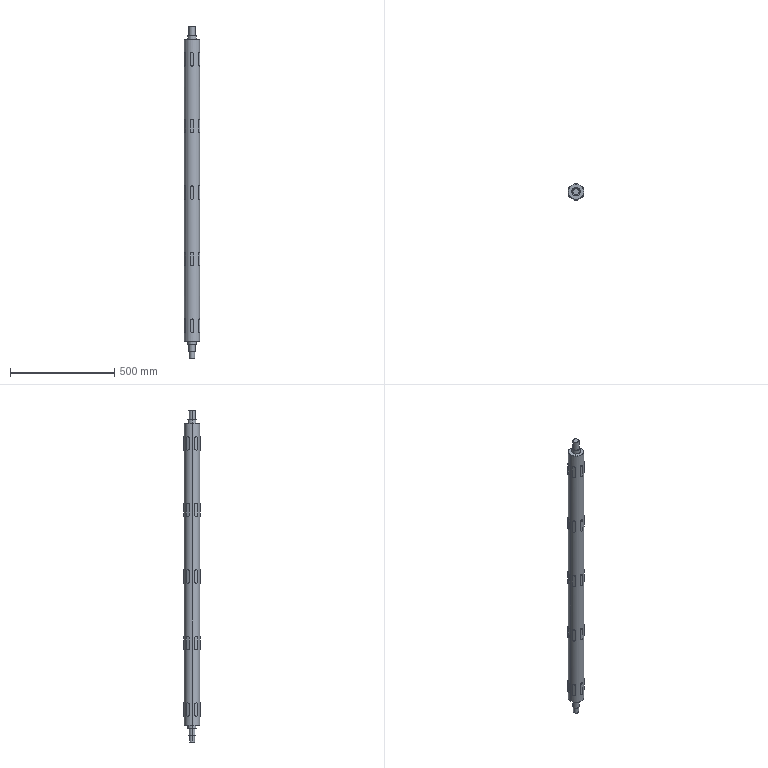Part | SolidWorks | features ICE 8, Chamfer 2, CirPattern 1, Extrusion 1, HoleWzd 1, LPattern 1 | 1 solid | 199 faces | box 76.782 x 80 x 1595 mm | volume 6439202 mm3 | plane 100 | cylinder 85 | cone 14 | commonest cylinder face diameters 15 x70 30 x4 40 x4 6.8 x2 25 x2 74 x2